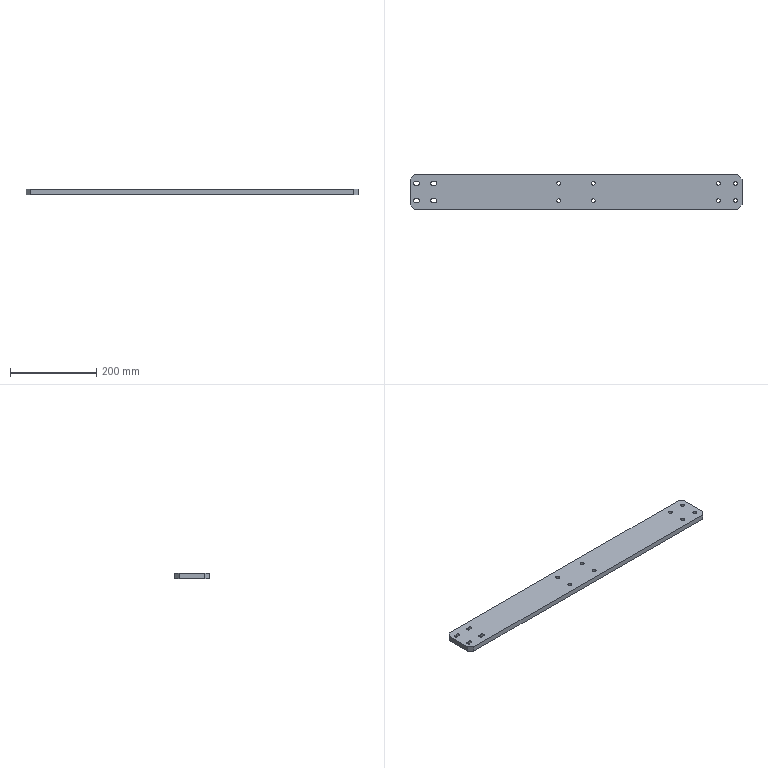Part | SolidWorks | features BaseBody 1 | 1 solid | 46 faces | box 770 x 80 x 12 mm | volume 725479 mm3 | cylinder 28 | plane 18 | commonest cylinder face diameters 9 x28
STEP:
#1=CARTESIAN_POINT('',(-363.,-20.,0.));
#2=VERTEX_POINT('',#1);
#3=CARTESIAN_POINT('',(-367.5,-15.5,0.));
#4=VERTEX_POINT('',#3);
#5=CARTESIAN_POINT('',(-367.5,-20.,0.));
#6=DIRECTION('',(0.,0.,1.));
#7=DIRECTION('',(1.,0.,0.));
#8=AXIS2_PLACEMENT_3D('',#5,#6,#7);
#9=CIRCLE('',#8,4.5);
#10=EDGE_CURVE('',#2,#4,#9,.T.);
#11=ORIENTED_EDGE('',*,*,#10,.F.);
#12=CARTESIAN_POINT('',(-363.,-20.,12.));
#13=VERTEX_POINT('',#12);
#14=CARTESIAN_POINT('',(-363.,-20.,0.));
#15=DIRECTION('',(0.,0.,1.));
#16=VECTOR('',#15,1000.);
#17=LINE('',#14,#16);
#18=EDGE_CURVE('',#2,#13,#17,.T.);
#19=ORIENTED_EDGE('',*,*,#18,.T.);
#20=CARTESIAN_POINT('',(-367.5,-15.5,12.));
#21=VERTEX_POINT('',#20);
#22=CARTESIAN_POINT('',(-367.5,-20.,12.));
#23=DIRECTION('',(0.,0.,1.));
#24=DIRECTION('',(1.,0.,0.));
#25=AXIS2_PLACEMENT_3D('',#22,#23,#24);
#26=CIRCLE('',#25,4.5);
#27=EDGE_CURVE('',#13,#21,#26,.T.);
#28=ORIENTED_EDGE('',*,*,#27,.T.);
#29=CARTESIAN_POINT('',(-367.5,-15.5,0.));
#30=DIRECTION('',(0.,0.,1.));
#31=VECTOR('',#30,1000.);
#32=LINE('',#29,#31);
#33=EDGE_CURVE('',#4,#21,#32,.T.);
#34=ORIENTED_EDGE('',*,*,#33,.F.);
#35=EDGE_LOOP('',(#11,#19,#28,#34));
#36=FACE_OUTER_BOUND('',#35,.T.);
#37=CARTESIAN_POINT('',(-367.5,-20.,0.));
#38=DIRECTION('',(0.,0.,1.));
#39=DIRECTION('',(1.,0.,0.));
#40=AXIS2_PLACEMENT_3D('',#37,#38,#39);
#41=CYLINDRICAL_SURFACE('',#40,4.5);
#42=ADVANCED_FACE('',(#36),#41,.F.);
#43=CARTESIAN_POINT('',(-323.,-20.,0.));
#44=VERTEX_POINT('',#43);
#45=CARTESIAN_POINT('',(-327.5,-15.5,0.));
#46=VERTEX_POINT('',#45);
#47=CARTESIAN_POINT('',(-327.5,-20.,0.));
#48=DIRECTION('',(0.,0.,1.));
#49=DIRECTION('',(1.,0.,0.));
#50=AXIS2_PLACEMENT_3D('',#47,#48,#49);
#51=CIRCLE('',#50,4.5);
#52=EDGE_CURVE('',#44,#46,#51,.T.);
#53=ORIENTED_EDGE('',*,*,#52,.F.);
#54=CARTESIAN_POINT('',(-323.,-20.,12.));
#55=VERTEX_POINT('',#54);
#56=CARTESIAN_POINT('',(-323.,-20.,0.));
#57=DIRECTION('',(0.,0.,1.));
#58=VECTOR('',#57,1000.);
#59=LINE('',#56,#58);
#60=EDGE_CURVE('',#44,#55,#59,.T.);
#61=ORIENTED_EDGE('',*,*,#60,.T.);
#62=CARTESIAN_POINT('',(-327.5,-15.5,12.));
#63=VERTEX_POINT('',#62);
#64=CARTESIAN_POINT('',(-327.5,-20.,12.));
#65=DIRECTION('',(0.,0.,1.));
#66=DIRECTION('',(1.,0.,0.));
#67=AXIS2_PLACEMENT_3D('',#64,#65,#66);
#68=CIRCLE('',#67,4.5);
#69=EDGE_CURVE('',#55,#63,#68,.T.);
#70=ORIENTED_EDGE('',*,*,#69,.T.);
#71=CARTESIAN_POINT('',(-327.5,-15.5,0.));
#72=DIRECTION('',(0.,0.,1.));
#73=VECTOR('',#72,1000.);
#74=LINE('',#71,#73);
#75=EDGE_CURVE('',#46,#63,#74,.T.);
#76=ORIENTED_EDGE('',*,*,#75,.F.);
#77=EDGE_LOOP('',(#53,#61,#70,#76));
#78=FACE_OUTER_BOUND('',#77,.T.);
#79=CARTESIAN_POINT('',(-327.5,-20.,0.));
#80=DIRECTION('',(0.,0.,1.));
#81=DIRECTION('',(1.,0.,0.));
#82=AXIS2_PLACEMENT_3D('',#79,#80,#81);
#83=CYLINDRICAL_SURFACE('',#82,4.5);
#84=ADVANCED_FACE('',(#78),#83,.F.);
#85=CARTESIAN_POINT('',(-323.,20.,0.));
#86=VERTEX_POINT('',#85);
#87=CARTESIAN_POINT('',(-327.5,24.5,0.));
#88=VERTEX_POINT('',#87);
#89=CARTESIAN_POINT('',(-327.5,20.,0.));
#90=DIRECTION('',(0.,0.,1.));
#91=DIRECTION('',(1.,0.,0.));
#92=AXIS2_PLACEMENT_3D('',#89,#90,#91);
#93=CIRCLE('',#92,4.5);
#94=EDGE_CURVE('',#86,#88,#93,.T.);
#95=ORIENTED_EDGE('',*,*,#94,.F.);
#96=CARTESIAN_POINT('',(-323.,20.,12.));
#97=VERTEX_POINT('',#96);
#98=CARTESIAN_POINT('',(-323.,20.,0.));
#99=DIRECTION('',(0.,0.,1.));
#100=VECTOR('',#99,1000.);
#101=LINE('',#98,#100);
#102=EDGE_CURVE('',#86,#97,#101,.T.);
#103=ORIENTED_EDGE('',*,*,#102,.T.);
#104=CARTESIAN_POINT('',(-327.5,24.5,12.));
#105=VERTEX_POINT('',#104);
#106=CARTESIAN_POINT('',(-327.5,20.,12.));
#107=DIRECTION('',(0.,0.,1.));
#108=DIRECTION('',(1.,0.,0.));
#109=AXIS2_PLACEMENT_3D('',#106,#107,#108);
#110=CIRCLE('',#109,4.5);
#111=EDGE_CURVE('',#97,#105,#110,.T.);
#112=ORIENTED_EDGE('',*,*,#111,.T.);
#113=CARTESIAN_POINT('',(-327.5,24.5,0.));
#114=DIRECTION('',(0.,0.,1.));
#115=VECTOR('',#114,1000.);
#116=LINE('',#113,#115);
#117=EDGE_CURVE('',#88,#105,#116,.T.);
#118=ORIENTED_EDGE('',*,*,#117,.F.);
#119=EDGE_LOOP('',(#95,#103,#112,#118));
#120=FACE_OUTER_BOUND('',#119,.T.);
#121=CARTESIAN_POINT('',(-327.5,20.,0.));
#122=DIRECTION('',(0.,0.,1.));
#123=DIRECTION('',(1.,0.,0.));
#124=AXIS2_PLACEMENT_3D('',#121,#122,#123);
#125=CYLINDRICAL_SURFACE('',#124,4.5);
#126=ADVANCED_FACE('',(#120),#125,.F.);
#127=CARTESIAN_POINT('',(-363.,20.,0.));
#128=VERTEX_POINT('',#127);
#129=CARTESIAN_POINT('',(-367.5,24.5,0.));
#130=VERTEX_POINT('',#129);
#131=CARTESIAN_POINT('',(-367.5,20.,0.));
#132=DIRECTION('',(0.,0.,1.));
#133=DIRECTION('',(1.,0.,0.));
#134=AXIS2_PLACEMENT_3D('',#131,#132,#133);
#135=CIRCLE('',#134,4.5);
#136=EDGE_CURVE('',#128,#130,#135,.T.);
#137=ORIENTED_EDGE('',*,*,#136,.F.);
#138=CARTESIAN_POINT('',(-363.,20.,12.));
#139=VERTEX_POINT('',#138);
#140=CARTESIAN_POINT('',(-363.,20.,0.));
#141=DIRECTION('',(0.,0.,1.));
#142=VECTOR('',#141,1000.);
#143=LINE('',#140,#142);
#144=EDGE_CURVE('',#128,#139,#143,.T.);
#145=ORIENTED_EDGE('',*,*,#144,.T.);
#146=CARTESIAN_POINT('',(-367.5,24.5,12.));
#147=VERTEX_POINT('',#146);
#148=CARTESIAN_POINT('',(-367.5,20.,12.));
#149=DIRECTION('',(0.,0.,1.));
#150=DIRECTION('',(1.,0.,0.));
#151=AXIS2_PLACEMENT_3D('',#148,#149,#150);
#152=CIRCLE('',#151,4.5);
#153=EDGE_CURVE('',#139,#147,#152,.T.);
#154=ORIENTED_EDGE('',*,*,#153,.T.);
#155=CARTESIAN_POINT('',(-367.5,24.5,0.));
#156=DIRECTION('',(0.,0.,1.));
#157=VECTOR('',#156,1000.);
#158=LINE('',#155,#157);
#159=EDGE_CURVE('',#130,#147,#158,.T.);
#160=ORIENTED_EDGE('',*,*,#159,.F.);
#161=EDGE_LOOP('',(#137,#145,#154,#160));
#162=FACE_OUTER_BOUND('',#161,.T.);
#163=CARTESIAN_POINT('',(-367.5,20.,0.));
#164=DIRECTION('',(0.,0.,1.));
#165=DIRECTION('',(1.,0.,0.));
#166=AXIS2_PLACEMENT_3D('',#163,#164,#165);
#167=CYLINDRICAL_SURFACE('',#166,4.5);
#168=ADVANCED_FACE('',(#162),#167,.F.);
#169=CARTESIAN_POINT('',(334.5,20.,0.));
#170=VERTEX_POINT('',#169);
#171=CARTESIAN_POINT('',(325.5,20.,0.));
#172=VERTEX_POINT('',#171);
#173=CARTESIAN_POINT('',(330.,20.,0.));
#174=DIRECTION('',(0.,0.,-1.));
#175=DIRECTION('',(-1.,0.,0.));
#176=AXIS2_PLACEMENT_3D('',#173,#174,#175);
#177=CIRCLE('',#176,4.5);
#178=EDGE_CURVE('',#170,#172,#177,.T.);
#179=ORIENTED_EDGE('',*,*,#178,.T.);
#180=CARTESIAN_POINT('',(325.5,20.,12.));
#181=VERTEX_POINT('',#180);
#182=CARTESIAN_POINT('',(325.5,20.,12.));
#183=DIRECTION('',(0.,0.,1.));
#184=VECTOR('',#183,1000.);
#185=LINE('',#182,#184);
#186=EDGE_CURVE('',#172,#181,#185,.T.);
#187=ORIENTED_EDGE('',*,*,#186,.T.);
#188=CARTESIAN_POINT('',(334.5,20.,12.));
#189=VERTEX_POINT('',#188);
#190=CARTESIAN_POINT('',(330.,20.,12.));
#191=DIRECTION('',(0.,0.,1.));
#192=DIRECTION('',(1.,0.,0.));
#193=AXIS2_PLACEMENT_3D('',#190,#191,#192);
#194=CIRCLE('',#193,4.5);
#195=EDGE_CURVE('',#181,#189,#194,.T.);
#196=ORIENTED_EDGE('',*,*,#195,.T.);
#197=CARTESIAN_POINT('',(334.5,20.,12.));
#198=DIRECTION('',(0.,0.,1.));
#199=VECTOR('',#198,1000.);
#200=LINE('',#197,#199);
#201=EDGE_CURVE('',#170,#189,#200,.T.);
#202=ORIENTED_EDGE('',*,*,#201,.F.);
#203=EDGE_LOOP('',(#179,#187,#196,#202));
#204=FACE_OUTER_BOUND('',#203,.T.);
#205=CARTESIAN_POINT('',(330.,20.,12.));
#206=DIRECTION('',(0.,0.,1.));
#207=DIRECTION('',(1.,0.,0.));
#208=AXIS2_PLACEMENT_3D('',#205,#206,#207);
#209=CYLINDRICAL_SURFACE('',#208,4.5);
#210=ADVANCED_FACE('',(#204),#209,.F.);
#211=CARTESIAN_POINT('',(374.5,20.,0.));
#212=VERTEX_POINT('',#211);
#213=CARTESIAN_POINT('',(365.5,20.,0.));
#214=VERTEX_POINT('',#213);
#215=CARTESIAN_POINT('',(370.,20.,0.));
#216=DIRECTION('',(0.,0.,-1.));
#217=DIRECTION('',(-1.,0.,0.));
#218=AXIS2_PLACEMENT_3D('',#215,#216,#217);
#219=CIRCLE('',#218,4.5);
#220=EDGE_CURVE('',#212,#214,#219,.T.);
#221=ORIENTED_EDGE('',*,*,#220,.T.);
#222=CARTESIAN_POINT('',(365.5,20.,12.));
#223=VERTEX_POINT('',#222);
#224=CARTESIAN_POINT('',(365.5,20.,12.));
#225=DIRECTION('',(0.,0.,1.));
#226=VECTOR('',#225,1000.);
#227=LINE('',#224,#226);
#228=EDGE_CURVE('',#214,#223,#227,.T.);
#229=ORIENTED_EDGE('',*,*,#228,.T.);
#230=CARTESIAN_POINT('',(374.5,20.,12.));
#231=VERTEX_POINT('',#230);
#232=CARTESIAN_POINT('',(370.,20.,12.));
#233=DIRECTION('',(0.,0.,1.));
#234=DIRECTION('',(1.,0.,0.));
#235=AXIS2_PLACEMENT_3D('',#232,#233,#234);
#236=CIRCLE('',#235,4.5);
#237=EDGE_CURVE('',#223,#231,#236,.T.);
#238=ORIENTED_EDGE('',*,*,#237,.T.);
#239=CARTESIAN_POINT('',(374.5,20.,12.));
#240=DIRECTION('',(0.,0.,1.));
#241=VECTOR('',#240,1000.);
#242=LINE('',#239,#241);
#243=EDGE_CURVE('',#212,#231,#242,.T.);
#244=ORIENTED_EDGE('',*,*,#243,.F.);
#245=EDGE_LOOP('',(#221,#229,#238,#244));
#246=FACE_OUTER_BOUND('',#245,.T.);
#247=CARTESIAN_POINT('',(370.,20.,12.));
#248=DIRECTION('',(0.,0.,1.));
#249=DIRECTION('',(1.,0.,0.));
#250=AXIS2_PLACEMENT_3D('',#247,#248,#249);
#251=CYLINDRICAL_SURFACE('',#250,4.5);
#252=ADVANCED_FACE('',(#246),#251,.F.);
#253=CARTESIAN_POINT('',(374.5,-20.,0.));
#254=VERTEX_POINT('',#253);
#255=CARTESIAN_POINT('',(365.5,-20.,0.));
#256=VERTEX_POINT('',#255);
#257=CARTESIAN_POINT('',(370.,-20.,0.));
#258=DIRECTION('',(0.,0.,-1.));
#259=DIRECTION('',(-1.,0.,0.));
#260=AXIS2_PLACEMENT_3D('',#257,#258,#259);
#261=CIRCLE('',#260,4.5);
#262=EDGE_CURVE('',#254,#256,#261,.T.);
#263=ORIENTED_EDGE('',*,*,#262,.T.);
#264=CARTESIAN_POINT('',(365.5,-20.,12.));
#265=VERTEX_POINT('',#264);
#266=CARTESIAN_POINT('',(365.5,-20.,12.));
#267=DIRECTION('',(0.,0.,1.));
#268=VECTOR('',#267,1000.);
#269=LINE('',#266,#268);
#270=EDGE_CURVE('',#256,#265,#269,.T.);
#271=ORIENTED_EDGE('',*,*,#270,.T.);
#272=CARTESIAN_POINT('',(374.5,-20.,12.));
#273=VERTEX_POINT('',#272);
#274=CARTESIAN_POINT('',(370.,-20.,12.));
#275=DIRECTION('',(0.,0.,1.));
#276=DIRECTION('',(1.,0.,0.));
#277=AXIS2_PLACEMENT_3D('',#274,#275,#276);
#278=CIRCLE('',#277,4.5);
#279=EDGE_CURVE('',#265,#273,#278,.T.);
#280=ORIENTED_EDGE('',*,*,#279,.T.);
#281=CARTESIAN_POINT('',(374.5,-20.,12.));
#282=DIRECTION('',(0.,0.,1.));
#283=VECTOR('',#282,1000.);
#284=LINE('',#281,#283);
#285=EDGE_CURVE('',#254,#273,#284,.T.);
#286=ORIENTED_EDGE('',*,*,#285,.F.);
#287=EDGE_LOOP('',(#263,#271,#280,#286));
#288=FACE_OUTER_BOUND('',#287,.T.);
#289=CARTESIAN_POINT('',(370.,-20.,12.));
#290=DIRECTION('',(0.,0.,1.));
#291=DIRECTION('',(1.,0.,0.));
#292=AXIS2_PLACEMENT_3D('',#289,#290,#291);
#293=CYLINDRICAL_SURFACE('',#292,4.5);
#294=ADVANCED_FACE('',(#288),#293,.F.);
#295=CARTESIAN_POINT('',(334.5,-20.,0.));
#296=VERTEX_POINT('',#295);
#297=CARTESIAN_POINT('',(325.5,-20.,0.));
#298=VERTEX_POINT('',#297);
#299=CARTESIAN_POINT('',(330.,-20.,0.));
#300=DIRECTION('',(0.,0.,-1.));
#301=DIRECTION('',(-1.,0.,0.));
#302=AXIS2_PLACEMENT_3D('',#299,#300,#301);
#303=CIRCLE('',#302,4.5);
#304=EDGE_CURVE('',#296,#298,#303,.T.);
#305=ORIENTED_EDGE('',*,*,#304,.T.);
#306=CARTESIAN_POINT('',(325.5,-20.,12.));
#307=VERTEX_POINT('',#306);
#308=CARTESIAN_POINT('',(325.5,-20.,12.));
#309=DIRECTION('',(0.,0.,1.));
#310=VECTOR('',#309,1000.);
#311=LINE('',#308,#310);
#312=EDGE_CURVE('',#298,#307,#311,.T.);
#313=ORIENTED_EDGE('',*,*,#312,.T.);
#314=CARTESIAN_POINT('',(334.5,-20.,12.));
#315=VERTEX_POINT('',#314);
#316=CARTESIAN_POINT('',(330.,-20.,12.));
#317=DIRECTION('',(0.,0.,1.));
#318=DIRECTION('',(1.,0.,0.));
#319=AXIS2_PLACEMENT_3D('',#316,#317,#318);
#320=CIRCLE('',#319,4.5);
#321=EDGE_CURVE('',#307,#315,#320,.T.);
#322=ORIENTED_EDGE('',*,*,#321,.T.);
#323=CARTESIAN_POINT('',(334.5,-20.,12.));
#324=DIRECTION('',(0.,0.,1.));
#325=VECTOR('',#324,1000.);
#326=LINE('',#323,#325);
#327=EDGE_CURVE('',#296,#315,#326,.T.);
#328=ORIENTED_EDGE('',*,*,#327,.F.);
#329=EDGE_LOOP('',(#305,#313,#322,#328));
#330=FACE_OUTER_BOUND('',#329,.T.);
#331=CARTESIAN_POINT('',(330.,-20.,12.));
#332=DIRECTION('',(0.,0.,1.));
#333=DIRECTION('',(1.,0.,0.));
#334=AXIS2_PLACEMENT_3D('',#331,#332,#333);
#335=CYLINDRICAL_SURFACE('',#334,4.5);
#336=ADVANCED_FACE('',(#330),#335,.F.);
#337=CARTESIAN_POINT('',(44.5,-20.,0.));
#338=VERTEX_POINT('',#337);
#339=CARTESIAN_POINT('',(35.5,-20.,0.));
#340=VERTEX_POINT('',#339);
#341=CARTESIAN_POINT('',(40.,-20.,0.));
#342=DIRECTION('',(0.,0.,-1.));
#343=DIRECTION('',(-1.,0.,0.));
#344=AXIS2_PLACEMENT_3D('',#341,#342,#343);
#345=CIRCLE('',#344,4.5);
#346=EDGE_CURVE('',#338,#340,#345,.T.);
#347=ORIENTED_EDGE('',*,*,#346,.T.);
#348=CARTESIAN_POINT('',(35.5,-20.,12.));
#349=VERTEX_POINT('',#348);
#350=CARTESIAN_POINT('',(35.5,-20.,12.));
#351=DIRECTION('',(0.,0.,1.));
#352=VECTOR('',#351,1000.);
#353=LINE('',#350,#352);
#354=EDGE_CURVE('',#340,#349,#353,.T.);
#355=ORIENTED_EDGE('',*,*,#354,.T.);
#356=CARTESIAN_POINT('',(44.5,-20.,12.));
#357=VERTEX_POINT('',#356);
#358=CARTESIAN_POINT('',(40.,-20.,12.));
#359=DIRECTION('',(0.,0.,1.));
#360=DIRECTION('',(1.,0.,0.));
#361=AXIS2_PLACEMENT_3D('',#358,#359,#360);
#362=CIRCLE('',#361,4.5);
#363=EDGE_CURVE('',#349,#357,#362,.T.);
#364=ORIENTED_EDGE('',*,*,#363,.T.);
#365=CARTESIAN_POINT('',(44.5,-20.,12.));
#366=DIRECTION('',(0.,0.,1.));
#367=VECTOR('',#366,1000.);
#368=LINE('',#365,#367);
#369=EDGE_CURVE('',#338,#357,#368,.T.);
#370=ORIENTED_EDGE('',*,*,#369,.F.);
#371=EDGE_LOOP('',(#347,#355,#364,#370));
#372=FACE_OUTER_BOUND('',#371,.T.);
#373=CARTESIAN_POINT('',(40.,-20.,12.));
#374=DIRECTION('',(0.,0.,1.));
#375=DIRECTION('',(1.,0.,0.));
#376=AXIS2_PLACEMENT_3D('',#373,#374,#375);
#377=CYLINDRICAL_SURFACE('',#376,4.5);
#378=ADVANCED_FACE('',(#372),#377,.F.);
#379=CARTESIAN_POINT('',(-35.5,20.,0.));
#380=VERTEX_POINT('',#379);
#381=CARTESIAN_POINT('',(-44.5,20.,0.));
#382=VERTEX_POINT('',#381);
#383=CARTESIAN_POINT('',(-40.,20.,0.));
#384=DIRECTION('',(0.,0.,-1.));
#385=DIRECTION('',(-1.,0.,0.));
#386=AXIS2_PLACEMENT_3D('',#383,#384,#385);
#387=CIRCLE('',#386,4.5);
#388=EDGE_CURVE('',#380,#382,#387,.T.);
#389=ORIENTED_EDGE('',*,*,#388,.T.);
#390=CARTESIAN_POINT('',(-44.5,20.,12.));
#391=VERTEX_POINT('',#390);
#392=CARTESIAN_POINT('',(-44.5,20.,12.));
#393=DIRECTION('',(0.,0.,1.));
#394=VECTOR('',#393,1000.);
#395=LINE('',#392,#394);
#396=EDGE_CURVE('',#382,#391,#395,.T.);
#397=ORIENTED_EDGE('',*,*,#396,.T.);
#398=CARTESIAN_POINT('',(-35.5,20.,12.));
#399=VERTEX_POINT('',#398);
#400=CARTESIAN_POINT('',(-40.,20.,12.));
#401=DIRECTION('',(0.,0.,1.));
#402=DIRECTION('',(1.,0.,0.));
#403=AXIS2_PLACEMENT_3D('',#400,#401,#402);
#404=CIRCLE('',#403,4.5);
#405=EDGE_CURVE('',#391,#399,#404,.T.);
#406=ORIENTED_EDGE('',*,*,#405,.T.);
#407=CARTESIAN_POINT('',(-35.5,20.,12.));
#408=DIRECTION('',(0.,0.,1.));
#409=VECTOR('',#408,1000.);
#410=LINE('',#407,#409);
#411=EDGE_CURVE('',#380,#399,#410,.T.);
#412=ORIENTED_EDGE('',*,*,#411,.F.);
#413=EDGE_LOOP('',(#389,#397,#406,#412));
#414=FACE_OUTER_BOUND('',#413,.T.);
#415=CARTESIAN_POINT('',(-40.,20.,12.));
#416=DIRECTION('',(0.,0.,1.));
#417=DIRECTION('',(1.,0.,0.));
#418=AXIS2_PLACEMENT_3D('',#415,#416,#417);
#419=CYLINDRICAL_SURFACE('',#418,4.5);
#420=ADVANCED_FACE('',(#414),#419,.F.);
#421=CARTESIAN_POINT('',(-35.5,-20.,0.));
#422=VERTEX_POINT('',#421);
#423=CARTESIAN_POINT('',(-44.5,-20.,0.));
#424=VERTEX_POINT('',#423);
#425=CARTESIAN_POINT('',(-40.,-20.,0.));
#426=DIRECTION('',(0.,0.,-1.));
#427=DIRECTION('',(-1.,0.,0.));
#428=AXIS2_PLACEMENT_3D('',#425,#426,#427);
#429=CIRCLE('',#428,4.5);
#430=EDGE_CURVE('',#422,#424,#429,.T.);
#431=ORIENTED_EDGE('',*,*,#430,.T.);
#432=CARTESIAN_POINT('',(-44.5,-20.,12.));
#433=VERTEX_POINT('',#432);
#434=CARTESIAN_POINT('',(-44.5,-20.,12.));
#435=DIRECTION('',(0.,0.,1.));
#436=VECTOR('',#435,1000.);
#437=LINE('',#434,#436);
#438=EDGE_CURVE('',#424,#433,#437,.T.);
#439=ORIENTED_EDGE('',*,*,#438,.T.);
#440=CARTESIAN_POINT('',(-35.5,-20.,12.));
#441=VERTEX_POINT('',#440);
#442=CARTESIAN_POINT('',(-40.,-20.,12.));
#443=DIRECTION('',(0.,0.,1.));
#444=DIRECTION('',(1.,0.,0.));
#445=AXIS2_PLACEMENT_3D('',#442,#443,#444);
#446=CIRCLE('',#445,4.5);
#447=EDGE_CURVE('',#433,#441,#446,.T.);
#448=ORIENTED_EDGE('',*,*,#447,.T.);
#449=CARTESIAN_POINT('',(-35.5,-20.,12.));
#450=DIRECTION('',(0.,0.,1.));
#451=VECTOR('',#450,1000.);
#452=LINE('',#449,#451);
#453=EDGE_CURVE('',#422,#441,#452,.T.);
#454=ORIENTED_EDGE('',*,*,#453,.F.);
#455=EDGE_LOOP('',(#431,#439,#448,#454));
#456=FACE_OUTER_BOUND('',#455,.T.);
#457=CARTESIAN_POINT('',(-40.,-20.,12.));
#458=DIRECTION('',(0.,0.,1.));
#459=DIRECTION('',(1.,0.,0.));
#460=AXIS2_PLACEMENT_3D('',#457,#458,#459);
#461=CYLINDRICAL_SURFACE('',#460,4.5);
#462=ADVANCED_FACE('',(#456),#461,.F.);
#463=CARTESIAN_POINT('',(44.5,20.,0.));
#464=VERTEX_POINT('',#463);
#465=CARTESIAN_POINT('',(35.5,20.,0.));
#466=VERTEX_POINT('',#465);
#467=CARTESIAN_POINT('',(40.,20.,0.));
#468=DIRECTION('',(0.,0.,-1.));
#469=DIRECTION('',(-1.,0.,0.));
#470=AXIS2_PLACEMENT_3D('',#467,#468,#469);
#471=CIRCLE('',#470,4.5);
#472=EDGE_CURVE('',#464,#466,#471,.T.);
#473=ORIENTED_EDGE('',*,*,#472,.T.);
#474=CARTESIAN_POINT('',(35.5,20.,12.));
#475=VERTEX_POINT('',#474);
#476=CARTESIAN_POINT('',(35.5,20.,12.));
#477=DIRECTION('',(0.,0.,1.));
#478=VECTOR('',#477,1000.);
#479=LINE('',#476,#478);
#480=EDGE_CURVE('',#466,#475,#479,.T.);
#481=ORIENTED_EDGE('',*,*,#480,.T.);
#482=CARTESIAN_POINT('',(44.5,20.,12.));
#483=VERTEX_POINT('',#482);
#484=CARTESIAN_POINT('',(40.,20.,12.));
#485=DIRECTION('',(0.,0.,1.));
#486=DIRECTION('',(1.,0.,0.));
#487=AXIS2_PLACEMENT_3D('',#484,#485,#486);
#488=CIRCLE('',#487,4.5);
#489=EDGE_CURVE('',#475,#483,#488,.T.);
#490=ORIENTED_EDGE('',*,*,#489,.T.);
#491=CARTESIAN_POINT('',(44.5,20.,12.));
#492=DIRECTION('',(0.,0.,1.));
#493=VECTOR('',#492,1000.);
#494=LINE('',#491,#493);
#495=EDGE_CURVE('',#464,#483,#494,.T.);
#496=ORIENTED_EDGE('',*,*,#495,.F.);
#497=EDGE_LOOP('',(#473,#481,#490,#496));
#498=FACE_OUTER_BOUND('',#497,.T.);
#499=CARTESIAN_POINT('',(40.,20.,12.));
#500=DIRECTION('',(0.,0.,1.));
#501=DIRECTION('',(1.,0.,0.));
#502=AXIS2_PLACEMENT_3D('',#499,#500,#501);
#503=CYLINDRICAL_SURFACE('',#502,4.5);
#504=ADVANCED_FACE('',(#498),#503,.F.);
#505=CARTESIAN_POINT('',(375.,40.,0.));
#506=VERTEX_POINT('',#505);
#507=CARTESIAN_POINT('',(-375.,40.,0.));
#508=VERTEX_POINT('',#507);
#509=CARTESIAN_POINT('',(-375.,40.,0.));
#510=DIRECTION('',(-1.,0.,0.));
#511=VECTOR('',#510,1000.);
#512=LINE('',#509,#511);
#513=EDGE_CURVE('',#506,#508,#512,.T.);
#514=ORIENTED_EDGE('',*,*,#513,.T.);
#515=CARTESIAN_POINT('',(-375.,40.,12.));
#516=VERTEX_POINT('',#515);
#517=CARTESIAN_POINT('',(-375.,40.,12.));
#518=DIRECTION('',(0.,0.,-1.));
#519=VECTOR('',#518,1000.);
#520=LINE('',#517,#519);
#521=EDGE_CURVE('',#516,#508,#520,.T.);
#522=ORIENTED_EDGE('',*,*,#521,.F.);
#523=CARTESIAN_POINT('',(375.,40.,12.));
#524=VERTEX_POINT('',#523);
#525=CARTESIAN_POINT('',(-375.,40.,12.));
#526=DIRECTION('',(-1.,0.,0.));
#527=VECTOR('',#526,1000.);
#528=LINE('',#525,#527);
#529=EDGE_CURVE('',#524,#516,#528,.T.);
#530=ORIENTED_EDGE('',*,*,#529,.F.);
#531=CARTESIAN_POINT('',(375.,40.,12.));
#532=DIRECTION('',(0.,0.,-1.));
#533=VECTOR('',#532,1000.);
#534=LINE('',#531,#533);
#535=EDGE_CURVE('',#524,#506,#534,.T.);
#536=ORIENTED_EDGE('',*,*,#535,.T.);
#537=EDGE_LOOP('',(#514,#522,#530,#536));
#538=FACE_OUTER_BOUND('',#537,.T.);
#539=CARTESIAN_POINT('',(-375.,40.,12.));
#540=DIRECTION('',(0.,-1.,0.));
#541=DIRECTION('',(0.,0.,-1.));
#542=AXIS2_PLACEMENT_3D('',#539,#540,#541);
#543=PLANE('',#542);
#544=ADVANCED_FACE('',(#538),#543,.F.);
#545=CARTESIAN_POINT('',(-385.,30.,0.));
#546=VERTEX_POINT('',#545);
#547=CARTESIAN_POINT('',(-385.,30.,0.));
#548=DIRECTION('',(-0.7071,-0.7071,0.));
#549=VECTOR('',#548,1000.);
#550=LINE('',#547,#549);
#551=EDGE_CURVE('',#508,#546,#550,.T.);
#552=ORIENTED_EDGE('',*,*,#551,.T.);
#553=CARTESIAN_POINT('',(-385.,30.,12.));
#554=VERTEX_POINT('',#553);
#555=CARTESIAN_POINT('',(-385.,30.,12.));
#556=DIRECTION('',(0.,0.,-1.));
#557=VECTOR('',#556,1000.);
#558=LINE('',#555,#557);
#559=EDGE_CURVE('',#554,#546,#558,.T.);
#560=ORIENTED_EDGE('',*,*,#559,.F.);
#561=CARTESIAN_POINT('',(-385.,30.,12.));
#562=DIRECTION('',(-0.7071,-0.7071,0.));
#563=VECTOR('',#562,1000.);
#564=LINE('',#561,#563);
#565=EDGE_CURVE('',#516,#554,#564,.T.);
#566=ORIENTED_EDGE('',*,*,#565,.F.);
#567=ORIENTED_EDGE('',*,*,#521,.T.);
#568=EDGE_LOOP('',(#552,#560,#566,#567));
#569=FACE_OUTER_BOUND('',#568,.T.);
#570=CARTESIAN_POINT('',(-385.,30.,12.));
#571=DIRECTION('',(0.7071,-0.7071,0.));
#572=DIRECTION('',(0.7071,0.7071,0.));
#573=AXIS2_PLACEMENT_3D('',#570,#571,#572);
#574=PLANE('',#573);
#575=ADVANCED_FACE('',(#569),#574,.F.);
#576=CARTESIAN_POINT('',(-385.,-30.,0.));
#577=VERTEX_POINT('',#576);
#578=CARTESIAN_POINT('',(-385.,30.,0.));
#579=DIRECTION('',(0.,-1.,0.));
#580=VECTOR('',#579,1000.);
#581=LINE('',#578,#580);
#582=EDGE_CURVE('',#546,#577,#581,.T.);
#583=ORIENTED_EDGE('',*,*,#582,.T.);
#584=CARTESIAN_POINT('',(-385.,-30.,12.));
#585=VERTEX_POINT('',#584);
#586=CARTESIAN_POINT('',(-385.,-30.,12.));
#587=DIRECTION('',(0.,0.,-1.));
#588=VECTOR('',#587,1000.);
#589=LINE('',#586,#588);
#590=EDGE_CURVE('',#585,#577,#589,.T.);
#591=ORIENTED_EDGE('',*,*,#590,.F.);
#592=CARTESIAN_POINT('',(-385.,30.,12.));
#593=DIRECTION('',(0.,-1.,0.));
#594=VECTOR('',#593,1000.);
#595=LINE('',#592,#594);
#596=EDGE_CURVE('',#554,#585,#595,.T.);
#597=ORIENTED_EDGE('',*,*,#596,.F.);
#598=ORIENTED_EDGE('',*,*,#559,.T.);
#599=EDGE_LOOP('',(#583,#591,#597,#598));
#600=FACE_OUTER_BOUND('',#599,.T.);
#601=CARTESIAN_POINT('',(-385.,30.,12.));
#602=DIRECTION('',(1.,0.,0.));
#603=DIRECTION('',(0.,0.,-1.));
#604=AXIS2_PLACEMENT_3D('',#601,#602,#603);
#605=PLANE('',#604);
#606=ADVANCED_FACE('',(#600),#605,.F.);
#607=CARTESIAN_POINT('',(-375.,-40.,0.));
#608=VERTEX_POINT('',#607);
#609=CARTESIAN_POINT('',(-385.,-30.,0.));
#610=DIRECTION('',(0.7071,-0.7071,0.));
#611=VECTOR('',#610,1000.);
#612=LINE('',#609,#611);
#613=EDGE_CURVE('',#577,#608,#612,.T.);
#614=ORIENTED_EDGE('',*,*,#613,.T.);
#615=CARTESIAN_POINT('',(-375.,-40.,12.));
#616=VERTEX_POINT('',#615);
#617=CARTESIAN_POINT('',(-375.,-40.,12.));
#618=DIRECTION('',(0.,0.,-1.));
#619=VECTOR('',#618,1000.);
#620=LINE('',#617,#619);
#621=EDGE_CURVE('',#616,#608,#620,.T.);
#622=ORIENTED_EDGE('',*,*,#621,.F.);
#623=CARTESIAN_POINT('',(-385.,-30.,12.));
#624=DIRECTION('',(0.7071,-0.7071,0.));
#625=VECTOR('',#624,1000.);
#626=LINE('',#623,#625);
#627=EDGE_CURVE('',#585,#616,#626,.T.);
#628=ORIENTED_EDGE('',*,*,#627,.F.);
#629=ORIENTED_EDGE('',*,*,#590,.T.);
#630=EDGE_LOOP('',(#614,#622,#628,#629));
#631=FACE_OUTER_BOUND('',#630,.T.);
#632=CARTESIAN_POINT('',(-385.,-30.,12.));
#633=DIRECTION('',(0.7071,0.7071,0.));
#634=DIRECTION('',(-0.7071,0.7071,0.));
#635=AXIS2_PLACEMENT_3D('',#632,#633,#634);
#636=PLANE('',#635);
#637=ADVANCED_FACE('',(#631),#636,.F.);
#638=CARTESIAN_POINT('',(375.,-40.,0.));
#639=VERTEX_POINT('',#638);
#640=CARTESIAN_POINT('',(-375.,-40.,0.));
#641=DIRECTION('',(1.,0.,0.));
#642=VECTOR('',#641,1000.);
#643=LINE('',#640,#642);
#644=EDGE_CURVE('',#608,#639,#643,.T.);
#645=ORIENTED_EDGE('',*,*,#644,.T.);
#646=CARTESIAN_POINT('',(375.,-40.,12.));
#647=VERTEX_POINT('',#646);
#648=CARTESIAN_POINT('',(375.,-40.,12.));
#649=DIRECTION('',(0.,0.,-1.));
#650=VECTOR('',#649,1000.);
#651=LINE('',#648,#650);
#652=EDGE_CURVE('',#647,#639,#651,.T.);
#653=ORIENTED_EDGE('',*,*,#652,.F.);
#654=CARTESIAN_POINT('',(-375.,-40.,12.));
#655=DIRECTION('',(1.,0.,0.));
#656=VECTOR('',#655,1000.);
#657=LINE('',#654,#656);
#658=EDGE_CURVE('',#616,#647,#657,.T.);
#659=ORIENTED_EDGE('',*,*,#658,.F.);
#660=ORIENTED_EDGE('',*,*,#621,.T.);
#661=EDGE_LOOP('',(#645,#653,#659,#660));
#662=FACE_OUTER_BOUND('',#661,.T.);
#663=CARTESIAN_POINT('',(-375.,-40.,12.));
#664=DIRECTION('',(0.,1.,0.));
#665=DIRECTION('',(0.,0.,1.));
#666=AXIS2_PLACEMENT_3D('',#663,#664,#665);
#667=PLANE('',#666);
#668=ADVANCED_FACE('',(#662),#667,.F.);
#669=CARTESIAN_POINT('',(385.,-30.,0.));
#670=VERTEX_POINT('',#669);
#671=CARTESIAN_POINT('',(375.,-40.,0.));
#672=DIRECTION('',(0.7071,0.7071,0.));
#673=VECTOR('',#672,1000.);
#674=LINE('',#671,#673);
#675=EDGE_CURVE('',#639,#670,#674,.T.);
#676=ORIENTED_EDGE('',*,*,#675,.T.);
#677=CARTESIAN_POINT('',(385.,-30.,12.));
#678=VERTEX_POINT('',#677);
#679=CARTESIAN_POINT('',(385.,-30.,12.));
#680=DIRECTION('',(0.,0.,-1.));
#681=VECTOR('',#680,1000.);
#682=LINE('',#679,#681);
#683=EDGE_CURVE('',#678,#670,#682,.T.);
#684=ORIENTED_EDGE('',*,*,#683,.F.);
#685=CARTESIAN_POINT('',(375.,-40.,12.));
#686=DIRECTION('',(0.7071,0.7071,0.));
#687=VECTOR('',#686,1000.);
#688=LINE('',#685,#687);
#689=EDGE_CURVE('',#647,#678,#688,.T.);
#690=ORIENTED_EDGE('',*,*,#689,.F.);
#691=ORIENTED_EDGE('',*,*,#652,.T.);
#692=EDGE_LOOP('',(#676,#684,#690,#691));
#693=FACE_OUTER_BOUND('',#692,.T.);
#694=CARTESIAN_POINT('',(375.,-40.,12.));
#695=DIRECTION('',(-0.7071,0.7071,0.));
#696=DIRECTION('',(-0.7071,-0.7071,0.));
#697=AXIS2_PLACEMENT_3D('',#694,#695,#696);
#698=PLANE('',#697);
#699=ADVANCED_FACE('',(#693),#698,.F.);
#700=CARTESIAN_POINT('',(385.,30.,0.));
#701=VERTEX_POINT('',#700);
#702=CARTESIAN_POINT('',(385.,30.,0.));
#703=DIRECTION('',(0.,1.,0.));
#704=VECTOR('',#703,1000.);
#705=LINE('',#702,#704);
#706=EDGE_CURVE('',#670,#701,#705,.T.);
#707=ORIENTED_EDGE('',*,*,#706,.T.);
#708=CARTESIAN_POINT('',(385.,30.,12.));
#709=VERTEX_POINT('',#708);
#710=CARTESIAN_POINT('',(385.,30.,12.));
#711=DIRECTION('',(0.,0.,-1.));
#712=VECTOR('',#711,1000.);
#713=LINE('',#710,#712);
#714=EDGE_CURVE('',#709,#701,#713,.T.);
#715=ORIENTED_EDGE('',*,*,#714,.F.);
#716=CARTESIAN_POINT('',(385.,30.,12.));
#717=DIRECTION('',(0.,1.,0.));
#718=VECTOR('',#717,1000.);
#719=LINE('',#716,#718);
#720=EDGE_CURVE('',#678,#709,#719,.T.);
#721=ORIENTED_EDGE('',*,*,#720,.F.);
#722=ORIENTED_EDGE('',*,*,#683,.T.);
#723=EDGE_LOOP('',(#707,#715,#721,#722));
#724=FACE_OUTER_BOUND('',#723,.T.);
#725=CARTESIAN_POINT('',(385.,30.,12.));
#726=DIRECTION('',(-1.,0.,0.));
#727=DIRECTION('',(0.,0.,1.));
#728=AXIS2_PLACEMENT_3D('',#725,#726,#727);
#729=PLANE('',#728);
#730=ADVANCED_FACE('',(#724),#729,.F.);
#731=CARTESIAN_POINT('',(375.,40.,0.));
#732=DIRECTION('',(-0.7071,0.7071,0.));
#733=VECTOR('',#732,1000.);
#734=LINE('',#731,#733);
#735=EDGE_CURVE('',#701,#506,#734,.T.);
#736=ORIENTED_EDGE('',*,*,#735,.T.);
#737=ORIENTED_EDGE('',*,*,#535,.F.);
#738=CARTESIAN_POINT('',(375.,40.,12.));
#739=DIRECTION('',(-0.7071,0.7071,0.));
#740=VECTOR('',#739,1000.);
#741=LINE('',#738,#740);
#742=EDGE_CURVE('',#709,#524,#741,.T.);
#743=ORIENTED_EDGE('',*,*,#742,.F.);
#744=ORIENTED_EDGE('',*,*,#714,.T.);
#745=EDGE_LOOP('',(#736,#737,#743,#744));
#746=FACE_OUTER_BOUND('',#745,.T.);
#747=CARTESIAN_POINT('',(375.,40.,12.));
#748=DIRECTION('',(-0.7071,-0.7071,0.));
#749=DIRECTION('',(0.7071,-0.7071,0.));
#750=AXIS2_PLACEMENT_3D('',#747,#748,#749);
#751=PLANE('',#750);
#752=ADVANCED_FACE('',(#746),#751,.F.);
#753=CARTESIAN_POINT('',(330.,20.,12.));
#754=DIRECTION('',(0.,0.,1.));
#755=DIRECTION('',(1.,0.,0.));
#756=AXIS2_PLACEMENT_3D('',#753,#754,#755);
#757=CIRCLE('',#756,4.5);
#758=EDGE_CURVE('',#189,#181,#757,.T.);
#759=ORIENTED_EDGE('',*,*,#758,.F.);
#760=ORIENTED_EDGE('',*,*,#195,.F.);
#761=EDGE_LOOP('',(#759,#760));
#762=FACE_BOUND('',#761,.T.);
#763=CARTESIAN_POINT('',(370.,20.,12.));
#764=DIRECTION('',(0.,0.,1.));
#765=DIRECTION('',(1.,0.,0.));
#766=AXIS2_PLACEMENT_3D('',#763,#764,#765);
#767=CIRCLE('',#766,4.5);
#768=EDGE_CURVE('',#231,#223,#767,.T.);
#769=ORIENTED_EDGE('',*,*,#768,.F.);
#770=ORIENTED_EDGE('',*,*,#237,.F.);
#771=EDGE_LOOP('',(#769,#770));
#772=FACE_BOUND('',#771,.T.);
#773=CARTESIAN_POINT('',(370.,-20.,12.));
#774=DIRECTION('',(0.,0.,1.));
#775=DIRECTION('',(1.,0.,0.));
#776=AXIS2_PLACEMENT_3D('',#773,#774,#775);
#777=CIRCLE('',#776,4.5);
#778=EDGE_CURVE('',#273,#265,#777,.T.);
#779=ORIENTED_EDGE('',*,*,#778,.F.);
#780=ORIENTED_EDGE('',*,*,#279,.F.);
#781=EDGE_LOOP('',(#779,#780));
#782=FACE_BOUND('',#781,.T.);
#783=CARTESIAN_POINT('',(330.,-20.,12.));
#784=DIRECTION('',(0.,0.,1.));
#785=DIRECTION('',(1.,0.,0.));
#786=AXIS2_PLACEMENT_3D('',#783,#784,#785);
#787=CIRCLE('',#786,4.5);
#788=EDGE_CURVE('',#315,#307,#787,.T.);
#789=ORIENTED_EDGE('',*,*,#788,.F.);
#790=ORIENTED_EDGE('',*,*,#321,.F.);
#791=EDGE_LOOP('',(#789,#790));
#792=FACE_BOUND('',#791,.T.);
#793=CARTESIAN_POINT('',(-372.5,15.5,12.));
#794=VERTEX_POINT('',#793);
#795=CARTESIAN_POINT('',(-367.5,15.5,12.));
#796=VERTEX_POINT('',#795);
#797=CARTESIAN_POINT('',(-372.5,15.5,12.));
#798=DIRECTION('',(1.,0.,0.));
#799=VECTOR('',#798,1000.);
#800=LINE('',#797,#799);
#801=EDGE_CURVE('',#794,#796,#800,.T.);
#802=ORIENTED_EDGE('',*,*,#801,.F.);
#803=CARTESIAN_POINT('',(-372.5,24.5,12.));
#804=VERTEX_POINT('',#803);
#805=CARTESIAN_POINT('',(-372.5,20.,12.));
#806=DIRECTION('',(0.,0.,1.));
#807=DIRECTION('',(1.,0.,0.));
#808=AXIS2_PLACEMENT_3D('',#805,#806,#807);
#809=CIRCLE('',#808,4.5);
#810=EDGE_CURVE('',#804,#794,#809,.T.);
#811=ORIENTED_EDGE('',*,*,#810,.F.);
#812=CARTESIAN_POINT('',(-372.5,24.5,12.));
#813=DIRECTION('',(-1.,0.,0.));
#814=VECTOR('',#813,1000.);
#815=LINE('',#812,#814);
#816=EDGE_CURVE('',#147,#804,#815,.T.);
#817=ORIENTED_EDGE('',*,*,#816,.F.);
#818=ORIENTED_EDGE('',*,*,#153,.F.);
#819=CARTESIAN_POINT('',(-367.5,20.,12.));
#820=DIRECTION('',(0.,0.,1.));
#821=DIRECTION('',(1.,0.,0.));
#822=AXIS2_PLACEMENT_3D('',#819,#820,#821);
#823=CIRCLE('',#822,4.5);
#824=EDGE_CURVE('',#796,#139,#823,.T.);
#825=ORIENTED_EDGE('',*,*,#824,.F.);
#826=EDGE_LOOP('',(#802,#811,#817,#818,#825));
#827=FACE_BOUND('',#826,.T.);
#828=CARTESIAN_POINT('',(-332.5,15.5,12.));
#829=VERTEX_POINT('',#828);
#830=CARTESIAN_POINT('',(-327.5,15.5,12.));
#831=VERTEX_POINT('',#830);
#832=CARTESIAN_POINT('',(-332.5,15.5,12.));
#833=DIRECTION('',(1.,0.,0.));
#834=VECTOR('',#833,1000.);
#835=LINE('',#832,#834);
#836=EDGE_CURVE('',#829,#831,#835,.T.);
#837=ORIENTED_EDGE('',*,*,#836,.F.);
#838=CARTESIAN_POINT('',(-332.5,24.5,12.));
#839=VERTEX_POINT('',#838);
#840=CARTESIAN_POINT('',(-332.5,20.,12.));
#841=DIRECTION('',(0.,0.,1.));
#842=DIRECTION('',(1.,0.,0.));
#843=AXIS2_PLACEMENT_3D('',#840,#841,#842);
#844=CIRCLE('',#843,4.5);
#845=EDGE_CURVE('',#839,#829,#844,.T.);
#846=ORIENTED_EDGE('',*,*,#845,.F.);
#847=CARTESIAN_POINT('',(-332.5,24.5,12.));
#848=DIRECTION('',(-1.,0.,0.));
#849=VECTOR('',#848,1000.);
#850=LINE('',#847,#849);
#851=EDGE_CURVE('',#105,#839,#850,.T.);
#852=ORIENTED_EDGE('',*,*,#851,.F.);
#853=ORIENTED_EDGE('',*,*,#111,.F.);
#854=CARTESIAN_POINT('',(-327.5,20.,12.));
#855=DIRECTION('',(0.,0.,1.));
#856=DIRECTION('',(1.,0.,0.));
#857=AXIS2_PLACEMENT_3D('',#854,#855,#856);
#858=CIRCLE('',#857,4.5);
#859=EDGE_CURVE('',#831,#97,#858,.T.);
#860=ORIENTED_EDGE('',*,*,#859,.F.);
#861=EDGE_LOOP('',(#837,#846,#852,#853,#860));
#862=FACE_BOUND('',#861,.T.);
#863=CARTESIAN_POINT('',(-332.5,-24.5,12.));
#864=VERTEX_POINT('',#863);
#865=CARTESIAN_POINT('',(-327.5,-24.5,12.));
#866=VERTEX_POINT('',#865);
#867=CARTESIAN_POINT('',(-332.5,-24.5,12.));
#868=DIRECTION('',(1.,0.,0.));
#869=VECTOR('',#868,1000.);
#870=LINE('',#867,#869);
#871=EDGE_CURVE('',#864,#866,#870,.T.);
#872=ORIENTED_EDGE('',*,*,#871,.F.);
#873=CARTESIAN_POINT('',(-332.5,-15.5,12.));
#874=VERTEX_POINT('',#873);
#875=CARTESIAN_POINT('',(-332.5,-20.,12.));
#876=DIRECTION('',(0.,0.,1.));
#877=DIRECTION('',(1.,0.,0.));
#878=AXIS2_PLACEMENT_3D('',#875,#876,#877);
#879=CIRCLE('',#878,4.5);
#880=EDGE_CURVE('',#874,#864,#879,.T.);
#881=ORIENTED_EDGE('',*,*,#880,.F.);
#882=CARTESIAN_POINT('',(-332.5,-15.5,12.));
#883=DIRECTION('',(-1.,0.,0.));
#884=VECTOR('',#883,1000.);
#885=LINE('',#882,#884);
#886=EDGE_CURVE('',#63,#874,#885,.T.);
#887=ORIENTED_EDGE('',*,*,#886,.F.);
#888=ORIENTED_EDGE('',*,*,#69,.F.);
#889=CARTESIAN_POINT('',(-327.5,-20.,12.));
#890=DIRECTION('',(0.,0.,1.));
#891=DIRECTION('',(1.,0.,0.));
#892=AXIS2_PLACEMENT_3D('',#889,#890,#891);
#893=CIRCLE('',#892,4.5);
#894=EDGE_CURVE('',#866,#55,#893,.T.);
#895=ORIENTED_EDGE('',*,*,#894,.F.);
#896=EDGE_LOOP('',(#872,#881,#887,#888,#895));
#897=FACE_BOUND('',#896,.T.);
#898=CARTESIAN_POINT('',(-372.5,-24.5,12.));
#899=VERTEX_POINT('',#898);
#900=CARTESIAN_POINT('',(-367.5,-24.5,12.));
#901=VERTEX_POINT('',#900);
#902=CARTESIAN_POINT('',(-372.5,-24.5,12.));
#903=DIRECTION('',(1.,0.,0.));
#904=VECTOR('',#903,1000.);
#905=LINE('',#902,#904);
#906=EDGE_CURVE('',#899,#901,#905,.T.);
#907=ORIENTED_EDGE('',*,*,#906,.F.);
#908=CARTESIAN_POINT('',(-372.5,-15.5,12.));
#909=VERTEX_POINT('',#908);
#910=CARTESIAN_POINT('',(-372.5,-20.,12.));
#911=DIRECTION('',(0.,0.,1.));
#912=DIRECTION('',(1.,0.,0.));
#913=AXIS2_PLACEMENT_3D('',#910,#911,#912);
#914=CIRCLE('',#913,4.5);
#915=EDGE_CURVE('',#909,#899,#914,.T.);
#916=ORIENTED_EDGE('',*,*,#915,.F.);
#917=CARTESIAN_POINT('',(-372.5,-15.5,12.));
#918=DIRECTION('',(-1.,0.,0.));
#919=VECTOR('',#918,1000.);
#920=LINE('',#917,#919);
#921=EDGE_CURVE('',#21,#909,#920,.T.);
#922=ORIENTED_EDGE('',*,*,#921,.F.);
#923=ORIENTED_EDGE('',*,*,#27,.F.);
#924=CARTESIAN_POINT('',(-367.5,-20.,12.));
#925=DIRECTION('',(0.,0.,1.));
#926=DIRECTION('',(1.,0.,0.));
#927=AXIS2_PLACEMENT_3D('',#924,#925,#926);
#928=CIRCLE('',#927,4.5);
#929=EDGE_CURVE('',#901,#13,#928,.T.);
#930=ORIENTED_EDGE('',*,*,#929,.F.);
#931=EDGE_LOOP('',(#907,#916,#922,#923,#930));
#932=FACE_BOUND('',#931,.T.);
#933=CARTESIAN_POINT('',(40.,-20.,12.));
#934=DIRECTION('',(0.,0.,1.));
#935=DIRECTION('',(1.,0.,0.));
#936=AXIS2_PLACEMENT_3D('',#933,#934,#935);
#937=CIRCLE('',#936,4.5);
#938=EDGE_CURVE('',#357,#349,#937,.T.);
#939=ORIENTED_EDGE('',*,*,#938,.F.);
#940=ORIENTED_EDGE('',*,*,#363,.F.);
#941=EDGE_LOOP('',(#939,#940));
#942=FACE_BOUND('',#941,.T.);
#943=CARTESIAN_POINT('',(-40.,20.,12.));
#944=DIRECTION('',(0.,0.,1.));
#945=DIRECTION('',(1.,0.,0.));
#946=AXIS2_PLACEMENT_3D('',#943,#944,#945);
#947=CIRCLE('',#946,4.5);
#948=EDGE_CURVE('',#399,#391,#947,.T.);
#949=ORIENTED_EDGE('',*,*,#948,.F.);
#950=ORIENTED_EDGE('',*,*,#405,.F.);
#951=EDGE_LOOP('',(#949,#950));
#952=FACE_BOUND('',#951,.T.);
#953=CARTESIAN_POINT('',(-40.,-20.,12.));
#954=DIRECTION('',(0.,0.,1.));
#955=DIRECTION('',(1.,0.,0.));
#956=AXIS2_PLACEMENT_3D('',#953,#954,#955);
#957=CIRCLE('',#956,4.5);
#958=EDGE_CURVE('',#441,#433,#957,.T.);
#959=ORIENTED_EDGE('',*,*,#958,.F.);
#960=ORIENTED_EDGE('',*,*,#447,.F.);
#961=EDGE_LOOP('',(#959,#960));
#962=FACE_BOUND('',#961,.T.);
#963=CARTESIAN_POINT('',(40.,20.,12.));
#964=DIRECTION('',(0.,0.,1.));
#965=DIRECTION('',(1.,0.,0.));
#966=AXIS2_PLACEMENT_3D('',#963,#964,#965);
#967=CIRCLE('',#966,4.5);
#968=EDGE_CURVE('',#483,#475,#967,.T.);
#969=ORIENTED_EDGE('',*,*,#968,.F.);
#970=ORIENTED_EDGE('',*,*,#489,.F.);
#971=EDGE_LOOP('',(#969,#970));
#972=FACE_BOUND('',#971,.T.);
#973=ORIENTED_EDGE('',*,*,#529,.T.);
#974=ORIENTED_EDGE('',*,*,#565,.T.);
#975=ORIENTED_EDGE('',*,*,#596,.T.);
#976=ORIENTED_EDGE('',*,*,#627,.T.);
#977=ORIENTED_EDGE('',*,*,#658,.T.);
#978=ORIENTED_EDGE('',*,*,#689,.T.);
#979=ORIENTED_EDGE('',*,*,#720,.T.);
#980=ORIENTED_EDGE('',*,*,#742,.T.);
#981=EDGE_LOOP('',(#973,#974,#975,#976,#977,#978,#979,#980));
#982=FACE_OUTER_BOUND('',#981,.T.);
#983=CARTESIAN_POINT('',(0.,0.,12.));
#984=DIRECTION('',(0.,0.,-1.));
#985=DIRECTION('',(-1.,0.,0.));
#986=AXIS2_PLACEMENT_3D('',#983,#984,#985);
#987=PLANE('',#986);
#988=ADVANCED_FACE('',(#762,#772,#782,#792,#827,#862,#897,#932,#942,#952,#962,#972,#982),#987,.F.);
#989=CARTESIAN_POINT('',(-372.5,-15.5,0.));
#990=VERTEX_POINT('',#989);
#991=CARTESIAN_POINT('',(-372.5,-24.5,0.));
#992=VERTEX_POINT('',#991);
#993=CARTESIAN_POINT('',(-372.5,-20.,0.));
#994=DIRECTION('',(0.,0.,1.));
#995=DIRECTION('',(1.,0.,0.));
#996=AXIS2_PLACEMENT_3D('',#993,#994,#995);
#997=CIRCLE('',#996,4.5);
#998=EDGE_CURVE('',#990,#992,#997,.T.);
#999=ORIENTED_EDGE('',*,*,#998,.T.);
#1000=CARTESIAN_POINT('',(-367.5,-24.5,0.));
#1001=VERTEX_POINT('',#1000);
#1002=CARTESIAN_POINT('',(-372.5,-24.5,0.));
#1003=DIRECTION('',(1.,0.,0.));
#1004=VECTOR('',#1003,1000.);
#1005=LINE('',#1002,#1004);
#1006=EDGE_CURVE('',#992,#1001,#1005,.T.);
#1007=ORIENTED_EDGE('',*,*,#1006,.T.);
#1008=CARTESIAN_POINT('',(-367.5,-20.,0.));
#1009=DIRECTION('',(0.,0.,1.));
#1010=DIRECTION('',(1.,0.,0.));
#1011=AXIS2_PLACEMENT_3D('',#1008,#1009,#1010);
#1012=CIRCLE('',#1011,4.5);
#1013=EDGE_CURVE('',#1001,#2,#1012,.T.);
#1014=ORIENTED_EDGE('',*,*,#1013,.T.);
#1015=ORIENTED_EDGE('',*,*,#10,.T.);
#1016=CARTESIAN_POINT('',(-372.5,-15.5,0.));
#1017=DIRECTION('',(-1.,0.,0.));
#1018=VECTOR('',#1017,1000.);
#1019=LINE('',#1016,#1018);
#1020=EDGE_CURVE('',#4,#990,#1019,.T.);
#1021=ORIENTED_EDGE('',*,*,#1020,.T.);
#1022=EDGE_LOOP('',(#999,#1007,#1014,#1015,#1021));
#1023=FACE_BOUND('',#1022,.T.);
#1024=CARTESIAN_POINT('',(-332.5,-15.5,0.));
#1025=VERTEX_POINT('',#1024);
#1026=CARTESIAN_POINT('',(-332.5,-24.5,0.));
#1027=VERTEX_POINT('',#1026);
#1028=CARTESIAN_POINT('',(-332.5,-20.,0.));
#1029=DIRECTION('',(0.,0.,1.));
#1030=DIRECTION('',(1.,0.,0.));
#1031=AXIS2_PLACEMENT_3D('',#1028,#1029,#1030);
#1032=CIRCLE('',#1031,4.5);
#1033=EDGE_CURVE('',#1025,#1027,#1032,.T.);
#1034=ORIENTED_EDGE('',*,*,#1033,.T.);
#1035=CARTESIAN_POINT('',(-327.5,-24.5,0.));
#1036=VERTEX_POINT('',#1035);
#1037=CARTESIAN_POINT('',(-332.5,-24.5,0.));
#1038=DIRECTION('',(1.,0.,0.));
#1039=VECTOR('',#1038,1000.);
#1040=LINE('',#1037,#1039);
#1041=EDGE_CURVE('',#1027,#1036,#1040,.T.);
#1042=ORIENTED_EDGE('',*,*,#1041,.T.);
#1043=CARTESIAN_POINT('',(-327.5,-20.,0.));
#1044=DIRECTION('',(0.,0.,1.));
#1045=DIRECTION('',(1.,0.,0.));
#1046=AXIS2_PLACEMENT_3D('',#1043,#1044,#1045);
#1047=CIRCLE('',#1046,4.5);
#1048=EDGE_CURVE('',#1036,#44,#1047,.T.);
#1049=ORIENTED_EDGE('',*,*,#1048,.T.);
#1050=ORIENTED_EDGE('',*,*,#52,.T.);
#1051=CARTESIAN_POINT('',(-332.5,-15.5,0.));
#1052=DIRECTION('',(-1.,0.,0.));
#1053=VECTOR('',#1052,1000.);
#1054=LINE('',#1051,#1053);
#1055=EDGE_CURVE('',#46,#1025,#1054,.T.);
#1056=ORIENTED_EDGE('',*,*,#1055,.T.);
#1057=EDGE_LOOP('',(#1034,#1042,#1049,#1050,#1056));
#1058=FACE_BOUND('',#1057,.T.);
#1059=CARTESIAN_POINT('',(-332.5,24.5,0.));
#1060=VERTEX_POINT('',#1059);
#1061=CARTESIAN_POINT('',(-332.5,15.5,0.));
#1062=VERTEX_POINT('',#1061);
#1063=CARTESIAN_POINT('',(-332.5,20.,0.));
#1064=DIRECTION('',(0.,0.,1.));
#1065=DIRECTION('',(1.,0.,0.));
#1066=AXIS2_PLACEMENT_3D('',#1063,#1064,#1065);
#1067=CIRCLE('',#1066,4.5);
#1068=EDGE_CURVE('',#1060,#1062,#1067,.T.);
#1069=ORIENTED_EDGE('',*,*,#1068,.T.);
#1070=CARTESIAN_POINT('',(-327.5,15.5,0.));
#1071=VERTEX_POINT('',#1070);
#1072=CARTESIAN_POINT('',(-332.5,15.5,0.));
#1073=DIRECTION('',(1.,0.,0.));
#1074=VECTOR('',#1073,1000.);
#1075=LINE('',#1072,#1074);
#1076=EDGE_CURVE('',#1062,#1071,#1075,.T.);
#1077=ORIENTED_EDGE('',*,*,#1076,.T.);
#1078=CARTESIAN_POINT('',(-327.5,20.,0.));
#1079=DIRECTION('',(0.,0.,1.));
#1080=DIRECTION('',(1.,0.,0.));
#1081=AXIS2_PLACEMENT_3D('',#1078,#1079,#1080);
#1082=CIRCLE('',#1081,4.5);
#1083=EDGE_CURVE('',#1071,#86,#1082,.T.);
#1084=ORIENTED_EDGE('',*,*,#1083,.T.);
#1085=ORIENTED_EDGE('',*,*,#94,.T.);
#1086=CARTESIAN_POINT('',(-332.5,24.5,0.));
#1087=DIRECTION('',(-1.,0.,0.));
#1088=VECTOR('',#1087,1000.);
#1089=LINE('',#1086,#1088);
#1090=EDGE_CURVE('',#88,#1060,#1089,.T.);
#1091=ORIENTED_EDGE('',*,*,#1090,.T.);
#1092=EDGE_LOOP('',(#1069,#1077,#1084,#1085,#1091));
#1093=FACE_BOUND('',#1092,.T.);
#1094=CARTESIAN_POINT('',(-372.5,24.5,0.));
#1095=VERTEX_POINT('',#1094);
#1096=CARTESIAN_POINT('',(-372.5,15.5,0.));
#1097=VERTEX_POINT('',#1096);
#1098=CARTESIAN_POINT('',(-372.5,20.,0.));
#1099=DIRECTION('',(0.,0.,1.));
#1100=DIRECTION('',(1.,0.,0.));
#1101=AXIS2_PLACEMENT_3D('',#1098,#1099,#1100);
#1102=CIRCLE('',#1101,4.5);
#1103=EDGE_CURVE('',#1095,#1097,#1102,.T.);
#1104=ORIENTED_EDGE('',*,*,#1103,.T.);
#1105=CARTESIAN_POINT('',(-367.5,15.5,0.));
#1106=VERTEX_POINT('',#1105);
#1107=CARTESIAN_POINT('',(-372.5,15.5,0.));
#1108=DIRECTION('',(1.,0.,0.));
#1109=VECTOR('',#1108,1000.);
#1110=LINE('',#1107,#1109);
#1111=EDGE_CURVE('',#1097,#1106,#1110,.T.);
#1112=ORIENTED_EDGE('',*,*,#1111,.T.);
#1113=CARTESIAN_POINT('',(-367.5,20.,0.));
#1114=DIRECTION('',(0.,0.,1.));
#1115=DIRECTION('',(1.,0.,0.));
#1116=AXIS2_PLACEMENT_3D('',#1113,#1114,#1115);
#1117=CIRCLE('',#1116,4.5);
#1118=EDGE_CURVE('',#1106,#128,#1117,.T.);
#1119=ORIENTED_EDGE('',*,*,#1118,.T.);
#1120=ORIENTED_EDGE('',*,*,#136,.T.);
#1121=CARTESIAN_POINT('',(-372.5,24.5,0.));
#1122=DIRECTION('',(-1.,0.,0.));
#1123=VECTOR('',#1122,1000.);
#1124=LINE('',#1121,#1123);
#1125=EDGE_CURVE('',#130,#1095,#1124,.T.);
#1126=ORIENTED_EDGE('',*,*,#1125,.T.);
#1127=EDGE_LOOP('',(#1104,#1112,#1119,#1120,#1126));
#1128=FACE_BOUND('',#1127,.T.);
#1129=ORIENTED_EDGE('',*,*,#178,.F.);
#1130=CARTESIAN_POINT('',(330.,20.,0.));
#1131=DIRECTION('',(0.,0.,-1.));
#1132=DIRECTION('',(-1.,0.,0.));
#1133=AXIS2_PLACEMENT_3D('',#1130,#1131,#1132);
#1134=CIRCLE('',#1133,4.5);
#1135=EDGE_CURVE('',#172,#170,#1134,.T.);
#1136=ORIENTED_EDGE('',*,*,#1135,.F.);
#1137=EDGE_LOOP('',(#1129,#1136));
#1138=FACE_BOUND('',#1137,.T.);
#1139=ORIENTED_EDGE('',*,*,#220,.F.);
#1140=CARTESIAN_POINT('',(370.,20.,0.));
#1141=DIRECTION('',(0.,0.,-1.));
#1142=DIRECTION('',(-1.,0.,0.));
#1143=AXIS2_PLACEMENT_3D('',#1140,#1141,#1142);
#1144=CIRCLE('',#1143,4.5);
#1145=EDGE_CURVE('',#214,#212,#1144,.T.);
#1146=ORIENTED_EDGE('',*,*,#1145,.F.);
#1147=EDGE_LOOP('',(#1139,#1146));
#1148=FACE_BOUND('',#1147,.T.);
#1149=ORIENTED_EDGE('',*,*,#262,.F.);
#1150=CARTESIAN_POINT('',(370.,-20.,0.));
#1151=DIRECTION('',(0.,0.,-1.));
#1152=DIRECTION('',(-1.,0.,0.));
#1153=AXIS2_PLACEMENT_3D('',#1150,#1151,#1152);
#1154=CIRCLE('',#1153,4.5);
#1155=EDGE_CURVE('',#256,#254,#1154,.T.);
#1156=ORIENTED_EDGE('',*,*,#1155,.F.);
#1157=EDGE_LOOP('',(#1149,#1156));
#1158=FACE_BOUND('',#1157,.T.);
#1159=ORIENTED_EDGE('',*,*,#304,.F.);
#1160=CARTESIAN_POINT('',(330.,-20.,0.));
#1161=DIRECTION('',(0.,0.,-1.));
#1162=DIRECTION('',(-1.,0.,0.));
#1163=AXIS2_PLACEMENT_3D('',#1160,#1161,#1162);
#1164=CIRCLE('',#1163,4.5);
#1165=EDGE_CURVE('',#298,#296,#1164,.T.);
#1166=ORIENTED_EDGE('',*,*,#1165,.F.);
#1167=EDGE_LOOP('',(#1159,#1166));
#1168=FACE_BOUND('',#1167,.T.);
#1169=ORIENTED_EDGE('',*,*,#346,.F.);
#1170=CARTESIAN_POINT('',(40.,-20.,0.));
#1171=DIRECTION('',(0.,0.,-1.));
#1172=DIRECTION('',(-1.,0.,0.));
#1173=AXIS2_PLACEMENT_3D('',#1170,#1171,#1172);
#1174=CIRCLE('',#1173,4.5);
#1175=EDGE_CURVE('',#340,#338,#1174,.T.);
#1176=ORIENTED_EDGE('',*,*,#1175,.F.);
#1177=EDGE_LOOP('',(#1169,#1176));
#1178=FACE_BOUND('',#1177,.T.);
#1179=ORIENTED_EDGE('',*,*,#388,.F.);
#1180=CARTESIAN_POINT('',(-40.,20.,0.));
#1181=DIRECTION('',(0.,0.,-1.));
#1182=DIRECTION('',(-1.,0.,0.));
#1183=AXIS2_PLACEMENT_3D('',#1180,#1181,#1182);
#1184=CIRCLE('',#1183,4.5);
#1185=EDGE_CURVE('',#382,#380,#1184,.T.);
#1186=ORIENTED_EDGE('',*,*,#1185,.F.);
#1187=EDGE_LOOP('',(#1179,#1186));
#1188=FACE_BOUND('',#1187,.T.);
#1189=ORIENTED_EDGE('',*,*,#430,.F.);
#1190=CARTESIAN_POINT('',(-40.,-20.,0.));
#1191=DIRECTION('',(0.,0.,-1.));
#1192=DIRECTION('',(-1.,0.,0.));
#1193=AXIS2_PLACEMENT_3D('',#1190,#1191,#1192);
#1194=CIRCLE('',#1193,4.5);
#1195=EDGE_CURVE('',#424,#422,#1194,.T.);
#1196=ORIENTED_EDGE('',*,*,#1195,.F.);
#1197=EDGE_LOOP('',(#1189,#1196));
#1198=FACE_BOUND('',#1197,.T.);
#1199=ORIENTED_EDGE('',*,*,#472,.F.);
#1200=CARTESIAN_POINT('',(40.,20.,0.));
#1201=DIRECTION('',(0.,0.,-1.));
#1202=DIRECTION('',(-1.,0.,0.));
#1203=AXIS2_PLACEMENT_3D('',#1200,#1201,#1202);
#1204=CIRCLE('',#1203,4.5);
#1205=EDGE_CURVE('',#466,#464,#1204,.T.);
#1206=ORIENTED_EDGE('',*,*,#1205,.F.);
#1207=EDGE_LOOP('',(#1199,#1206));
#1208=FACE_BOUND('',#1207,.T.);
#1209=ORIENTED_EDGE('',*,*,#513,.F.);
#1210=ORIENTED_EDGE('',*,*,#735,.F.);
#1211=ORIENTED_EDGE('',*,*,#706,.F.);
#1212=ORIENTED_EDGE('',*,*,#675,.F.);
#1213=ORIENTED_EDGE('',*,*,#644,.F.);
#1214=ORIENTED_EDGE('',*,*,#613,.F.);
#1215=ORIENTED_EDGE('',*,*,#582,.F.);
#1216=ORIENTED_EDGE('',*,*,#551,.F.);
#1217=EDGE_LOOP('',(#1209,#1210,#1211,#1212,#1213,#1214,#1215,#1216));
#1218=FACE_OUTER_BOUND('',#1217,.T.);
#1219=CARTESIAN_POINT('',(0.,0.,0.));
#1220=DIRECTION('',(0.,0.,-1.));
#1221=DIRECTION('',(-1.,0.,0.));
#1222=AXIS2_PLACEMENT_3D('',#1219,#1220,#1221);
#1223=PLANE('',#1222);
#1224=ADVANCED_FACE('',(#1023,#1058,#1093,#1128,#1138,#1148,#1158,#1168,#1178,#1188,#1198,#1208,#1218),#1223,.T.);
#1225=ORIENTED_EDGE('',*,*,#480,.F.);
#1226=ORIENTED_EDGE('',*,*,#1205,.T.);
#1227=ORIENTED_EDGE('',*,*,#495,.T.);
#1228=ORIENTED_EDGE('',*,*,#968,.T.);
#1229=EDGE_LOOP('',(#1225,#1226,#1227,#1228));
#1230=FACE_OUTER_BOUND('',#1229,.T.);
#1231=CARTESIAN_POINT('',(40.,20.,12.));
#1232=DIRECTION('',(0.,0.,1.));
#1233=DIRECTION('',(1.,0.,0.));
#1234=AXIS2_PLACEMENT_3D('',#1231,#1232,#1233);
#1235=CYLINDRICAL_SURFACE('',#1234,4.5);
#1236=ADVANCED_FACE('',(#1230),#1235,.F.);
#1237=ORIENTED_EDGE('',*,*,#438,.F.);
#1238=ORIENTED_EDGE('',*,*,#1195,.T.);
#1239=ORIENTED_EDGE('',*,*,#453,.T.);
#1240=ORIENTED_EDGE('',*,*,#958,.T.);
#1241=EDGE_LOOP('',(#1237,#1238,#1239,#1240));
#1242=FACE_OUTER_BOUND('',#1241,.T.);
#1243=CARTESIAN_POINT('',(-40.,-20.,12.));
#1244=DIRECTION('',(0.,0.,1.));
#1245=DIRECTION('',(1.,0.,0.));
#1246=AXIS2_PLACEMENT_3D('',#1243,#1244,#1245);
#1247=CYLINDRICAL_SURFACE('',#1246,4.5);
#1248=ADVANCED_FACE('',(#1242),#1247,.F.);
#1249=ORIENTED_EDGE('',*,*,#396,.F.);
#1250=ORIENTED_EDGE('',*,*,#1185,.T.);
#1251=ORIENTED_EDGE('',*,*,#411,.T.);
#1252=ORIENTED_EDGE('',*,*,#948,.T.);
#1253=EDGE_LOOP('',(#1249,#1250,#1251,#1252));
#1254=FACE_OUTER_BOUND('',#1253,.T.);
#1255=CARTESIAN_POINT('',(-40.,20.,12.));
#1256=DIRECTION('',(0.,0.,1.));
#1257=DIRECTION('',(1.,0.,0.));
#1258=AXIS2_PLACEMENT_3D('',#1255,#1256,#1257);
#1259=CYLINDRICAL_SURFACE('',#1258,4.5);
#1260=ADVANCED_FACE('',(#1254),#1259,.F.);
#1261=ORIENTED_EDGE('',*,*,#354,.F.);
#1262=ORIENTED_EDGE('',*,*,#1175,.T.);
#1263=ORIENTED_EDGE('',*,*,#369,.T.);
#1264=ORIENTED_EDGE('',*,*,#938,.T.);
#1265=EDGE_LOOP('',(#1261,#1262,#1263,#1264));
#1266=FACE_OUTER_BOUND('',#1265,.T.);
#1267=CARTESIAN_POINT('',(40.,-20.,12.));
#1268=DIRECTION('',(0.,0.,1.));
#1269=DIRECTION('',(1.,0.,0.));
#1270=AXIS2_PLACEMENT_3D('',#1267,#1268,#1269);
#1271=CYLINDRICAL_SURFACE('',#1270,4.5);
#1272=ADVANCED_FACE('',(#1266),#1271,.F.);
#1273=ORIENTED_EDGE('',*,*,#312,.F.);
#1274=ORIENTED_EDGE('',*,*,#1165,.T.);
#1275=ORIENTED_EDGE('',*,*,#327,.T.);
#1276=ORIENTED_EDGE('',*,*,#788,.T.);
#1277=EDGE_LOOP('',(#1273,#1274,#1275,#1276));
#1278=FACE_OUTER_BOUND('',#1277,.T.);
#1279=CARTESIAN_POINT('',(330.,-20.,12.));
#1280=DIRECTION('',(0.,0.,1.));
#1281=DIRECTION('',(1.,0.,0.));
#1282=AXIS2_PLACEMENT_3D('',#1279,#1280,#1281);
#1283=CYLINDRICAL_SURFACE('',#1282,4.5);
#1284=ADVANCED_FACE('',(#1278),#1283,.F.);
#1285=ORIENTED_EDGE('',*,*,#270,.F.);
#1286=ORIENTED_EDGE('',*,*,#1155,.T.);
#1287=ORIENTED_EDGE('',*,*,#285,.T.);
#1288=ORIENTED_EDGE('',*,*,#778,.T.);
#1289=EDGE_LOOP('',(#1285,#1286,#1287,#1288));
#1290=FACE_OUTER_BOUND('',#1289,.T.);
#1291=CARTESIAN_POINT('',(370.,-20.,12.));
#1292=DIRECTION('',(0.,0.,1.));
#1293=DIRECTION('',(1.,0.,0.));
#1294=AXIS2_PLACEMENT_3D('',#1291,#1292,#1293);
#1295=CYLINDRICAL_SURFACE('',#1294,4.5);
#1296=ADVANCED_FACE('',(#1290),#1295,.F.);
#1297=ORIENTED_EDGE('',*,*,#228,.F.);
#1298=ORIENTED_EDGE('',*,*,#1145,.T.);
#1299=ORIENTED_EDGE('',*,*,#243,.T.);
#1300=ORIENTED_EDGE('',*,*,#768,.T.);
#1301=EDGE_LOOP('',(#1297,#1298,#1299,#1300));
#1302=FACE_OUTER_BOUND('',#1301,.T.);
#1303=CARTESIAN_POINT('',(370.,20.,12.));
#1304=DIRECTION('',(0.,0.,1.));
#1305=DIRECTION('',(1.,0.,0.));
#1306=AXIS2_PLACEMENT_3D('',#1303,#1304,#1305);
#1307=CYLINDRICAL_SURFACE('',#1306,4.5);
#1308=ADVANCED_FACE('',(#1302),#1307,.F.);
#1309=ORIENTED_EDGE('',*,*,#186,.F.);
#1310=ORIENTED_EDGE('',*,*,#1135,.T.);
#1311=ORIENTED_EDGE('',*,*,#201,.T.);
#1312=ORIENTED_EDGE('',*,*,#758,.T.);
#1313=EDGE_LOOP('',(#1309,#1310,#1311,#1312));
#1314=FACE_OUTER_BOUND('',#1313,.T.);
#1315=CARTESIAN_POINT('',(330.,20.,12.));
#1316=DIRECTION('',(0.,0.,1.));
#1317=DIRECTION('',(1.,0.,0.));
#1318=AXIS2_PLACEMENT_3D('',#1315,#1316,#1317);
#1319=CYLINDRICAL_SURFACE('',#1318,4.5);
#1320=ADVANCED_FACE('',(#1314),#1319,.F.);
#1321=ORIENTED_EDGE('',*,*,#816,.T.);
#1322=CARTESIAN_POINT('',(-372.5,24.5,0.));
#1323=DIRECTION('',(0.,0.,1.));
#1324=VECTOR('',#1323,1000.);
#1325=LINE('',#1322,#1324);
#1326=EDGE_CURVE('',#1095,#804,#1325,.T.);
#1327=ORIENTED_EDGE('',*,*,#1326,.F.);
#1328=ORIENTED_EDGE('',*,*,#1125,.F.);
#1329=ORIENTED_EDGE('',*,*,#159,.T.);
#1330=EDGE_LOOP('',(#1321,#1327,#1328,#1329));
#1331=FACE_OUTER_BOUND('',#1330,.T.);
#1332=CARTESIAN_POINT('',(-372.5,24.5,0.));
#1333=DIRECTION('',(0.,1.,0.));
#1334=DIRECTION('',(0.,0.,1.));
#1335=AXIS2_PLACEMENT_3D('',#1332,#1333,#1334);
#1336=PLANE('',#1335);
#1337=ADVANCED_FACE('',(#1331),#1336,.F.);
#1338=ORIENTED_EDGE('',*,*,#801,.T.);
#1339=CARTESIAN_POINT('',(-367.5,15.5,0.));
#1340=DIRECTION('',(0.,0.,1.));
#1341=VECTOR('',#1340,1000.);
#1342=LINE('',#1339,#1341);
#1343=EDGE_CURVE('',#1106,#796,#1342,.T.);
#1344=ORIENTED_EDGE('',*,*,#1343,.F.);
#1345=ORIENTED_EDGE('',*,*,#1111,.F.);
#1346=CARTESIAN_POINT('',(-372.5,15.5,0.));
#1347=DIRECTION('',(0.,0.,1.));
#1348=VECTOR('',#1347,1000.);
#1349=LINE('',#1346,#1348);
#1350=EDGE_CURVE('',#1097,#794,#1349,.T.);
#1351=ORIENTED_EDGE('',*,*,#1350,.T.);
#1352=EDGE_LOOP('',(#1338,#1344,#1345,#1351));
#1353=FACE_OUTER_BOUND('',#1352,.T.);
#1354=CARTESIAN_POINT('',(-372.5,15.5,0.));
#1355=DIRECTION('',(0.,-1.,0.));
#1356=DIRECTION('',(1.,0.,0.));
#1357=AXIS2_PLACEMENT_3D('',#1354,#1355,#1356);
#1358=PLANE('',#1357);
#1359=ADVANCED_FACE('',(#1353),#1358,.F.);
#1360=ORIENTED_EDGE('',*,*,#810,.T.);
#1361=ORIENTED_EDGE('',*,*,#1350,.F.);
#1362=ORIENTED_EDGE('',*,*,#1103,.F.);
#1363=ORIENTED_EDGE('',*,*,#1326,.T.);
#1364=EDGE_LOOP('',(#1360,#1361,#1362,#1363));
#1365=FACE_OUTER_BOUND('',#1364,.T.);
#1366=CARTESIAN_POINT('',(-372.5,20.,0.));
#1367=DIRECTION('',(0.,0.,1.));
#1368=DIRECTION('',(1.,0.,0.));
#1369=AXIS2_PLACEMENT_3D('',#1366,#1367,#1368);
#1370=CYLINDRICAL_SURFACE('',#1369,4.5);
#1371=ADVANCED_FACE('',(#1365),#1370,.F.);
#1372=ORIENTED_EDGE('',*,*,#144,.F.);
#1373=ORIENTED_EDGE('',*,*,#1118,.F.);
#1374=ORIENTED_EDGE('',*,*,#1343,.T.);
#1375=ORIENTED_EDGE('',*,*,#824,.T.);
#1376=EDGE_LOOP('',(#1372,#1373,#1374,#1375));
#1377=FACE_OUTER_BOUND('',#1376,.T.);
#1378=CARTESIAN_POINT('',(-367.5,20.,0.));
#1379=DIRECTION('',(0.,0.,1.));
#1380=DIRECTION('',(1.,0.,0.));
#1381=AXIS2_PLACEMENT_3D('',#1378,#1379,#1380);
#1382=CYLINDRICAL_SURFACE('',#1381,4.5);
#1383=ADVANCED_FACE('',(#1377),#1382,.F.);
#1384=ORIENTED_EDGE('',*,*,#851,.T.);
#1385=CARTESIAN_POINT('',(-332.5,24.5,0.));
#1386=DIRECTION('',(0.,0.,1.));
#1387=VECTOR('',#1386,1000.);
#1388=LINE('',#1385,#1387);
#1389=EDGE_CURVE('',#1060,#839,#1388,.T.);
#1390=ORIENTED_EDGE('',*,*,#1389,.F.);
#1391=ORIENTED_EDGE('',*,*,#1090,.F.);
#1392=ORIENTED_EDGE('',*,*,#117,.T.);
#1393=EDGE_LOOP('',(#1384,#1390,#1391,#1392));
#1394=FACE_OUTER_BOUND('',#1393,.T.);
#1395=CARTESIAN_POINT('',(-332.5,24.5,0.));
#1396=DIRECTION('',(0.,1.,0.));
#1397=DIRECTION('',(0.,0.,1.));
#1398=AXIS2_PLACEMENT_3D('',#1395,#1396,#1397);
#1399=PLANE('',#1398);
#1400=ADVANCED_FACE('',(#1394),#1399,.F.);
#1401=ORIENTED_EDGE('',*,*,#836,.T.);
#1402=CARTESIAN_POINT('',(-327.5,15.5,0.));
#1403=DIRECTION('',(0.,0.,1.));
#1404=VECTOR('',#1403,1000.);
#1405=LINE('',#1402,#1404);
#1406=EDGE_CURVE('',#1071,#831,#1405,.T.);
#1407=ORIENTED_EDGE('',*,*,#1406,.F.);
#1408=ORIENTED_EDGE('',*,*,#1076,.F.);
#1409=CARTESIAN_POINT('',(-332.5,15.5,0.));
#1410=DIRECTION('',(0.,0.,1.));
#1411=VECTOR('',#1410,1000.);
#1412=LINE('',#1409,#1411);
#1413=EDGE_CURVE('',#1062,#829,#1412,.T.);
#1414=ORIENTED_EDGE('',*,*,#1413,.T.);
#1415=EDGE_LOOP('',(#1401,#1407,#1408,#1414));
#1416=FACE_OUTER_BOUND('',#1415,.T.);
#1417=CARTESIAN_POINT('',(-332.5,15.5,0.));
#1418=DIRECTION('',(0.,-1.,0.));
#1419=DIRECTION('',(1.,0.,0.));
#1420=AXIS2_PLACEMENT_3D('',#1417,#1418,#1419);
#1421=PLANE('',#1420);
#1422=ADVANCED_FACE('',(#1416),#1421,.F.);
#1423=ORIENTED_EDGE('',*,*,#845,.T.);
#1424=ORIENTED_EDGE('',*,*,#1413,.F.);
#1425=ORIENTED_EDGE('',*,*,#1068,.F.);
#1426=ORIENTED_EDGE('',*,*,#1389,.T.);
#1427=EDGE_LOOP('',(#1423,#1424,#1425,#1426));
#1428=FACE_OUTER_BOUND('',#1427,.T.);
#1429=CARTESIAN_POINT('',(-332.5,20.,0.));
#1430=DIRECTION('',(0.,0.,1.));
#1431=DIRECTION('',(1.,0.,0.));
#1432=AXIS2_PLACEMENT_3D('',#1429,#1430,#1431);
#1433=CYLINDRICAL_SURFACE('',#1432,4.5);
#1434=ADVANCED_FACE('',(#1428),#1433,.F.);
#1435=ORIENTED_EDGE('',*,*,#102,.F.);
#1436=ORIENTED_EDGE('',*,*,#1083,.F.);
#1437=ORIENTED_EDGE('',*,*,#1406,.T.);
#1438=ORIENTED_EDGE('',*,*,#859,.T.);
#1439=EDGE_LOOP('',(#1435,#1436,#1437,#1438));
#1440=FACE_OUTER_BOUND('',#1439,.T.);
#1441=CARTESIAN_POINT('',(-327.5,20.,0.));
#1442=DIRECTION('',(0.,0.,1.));
#1443=DIRECTION('',(1.,0.,0.));
#1444=AXIS2_PLACEMENT_3D('',#1441,#1442,#1443);
#1445=CYLINDRICAL_SURFACE('',#1444,4.5);
#1446=ADVANCED_FACE('',(#1440),#1445,.F.);
#1447=ORIENTED_EDGE('',*,*,#886,.T.);
#1448=CARTESIAN_POINT('',(-332.5,-15.5,0.));
#1449=DIRECTION('',(0.,0.,1.));
#1450=VECTOR('',#1449,1000.);
#1451=LINE('',#1448,#1450);
#1452=EDGE_CURVE('',#1025,#874,#1451,.T.);
#1453=ORIENTED_EDGE('',*,*,#1452,.F.);
#1454=ORIENTED_EDGE('',*,*,#1055,.F.);
#1455=ORIENTED_EDGE('',*,*,#75,.T.);
#1456=EDGE_LOOP('',(#1447,#1453,#1454,#1455));
#1457=FACE_OUTER_BOUND('',#1456,.T.);
#1458=CARTESIAN_POINT('',(-332.5,-15.5,0.));
#1459=DIRECTION('',(0.,1.,0.));
#1460=DIRECTION('',(-1.,0.,0.));
#1461=AXIS2_PLACEMENT_3D('',#1458,#1459,#1460);
#1462=PLANE('',#1461);
#1463=ADVANCED_FACE('',(#1457),#1462,.F.);
#1464=ORIENTED_EDGE('',*,*,#871,.T.);
#1465=CARTESIAN_POINT('',(-327.5,-24.5,0.));
#1466=DIRECTION('',(0.,0.,1.));
#1467=VECTOR('',#1466,1000.);
#1468=LINE('',#1465,#1467);
#1469=EDGE_CURVE('',#1036,#866,#1468,.T.);
#1470=ORIENTED_EDGE('',*,*,#1469,.F.);
#1471=ORIENTED_EDGE('',*,*,#1041,.F.);
#1472=CARTESIAN_POINT('',(-332.5,-24.5,0.));
#1473=DIRECTION('',(0.,0.,1.));
#1474=VECTOR('',#1473,1000.);
#1475=LINE('',#1472,#1474);
#1476=EDGE_CURVE('',#1027,#864,#1475,.T.);
#1477=ORIENTED_EDGE('',*,*,#1476,.T.);
#1478=EDGE_LOOP('',(#1464,#1470,#1471,#1477));
#1479=FACE_OUTER_BOUND('',#1478,.T.);
#1480=CARTESIAN_POINT('',(-332.5,-24.5,0.));
#1481=DIRECTION('',(0.,-1.,0.));
#1482=DIRECTION('',(0.,0.,-1.));
#1483=AXIS2_PLACEMENT_3D('',#1480,#1481,#1482);
#1484=PLANE('',#1483);
#1485=ADVANCED_FACE('',(#1479),#1484,.F.);
#1486=ORIENTED_EDGE('',*,*,#880,.T.);
#1487=ORIENTED_EDGE('',*,*,#1476,.F.);
#1488=ORIENTED_EDGE('',*,*,#1033,.F.);
#1489=ORIENTED_EDGE('',*,*,#1452,.T.);
#1490=EDGE_LOOP('',(#1486,#1487,#1488,#1489));
#1491=FACE_OUTER_BOUND('',#1490,.T.);
#1492=CARTESIAN_POINT('',(-332.5,-20.,0.));
#1493=DIRECTION('',(0.,0.,1.));
#1494=DIRECTION('',(1.,0.,0.));
#1495=AXIS2_PLACEMENT_3D('',#1492,#1493,#1494);
#1496=CYLINDRICAL_SURFACE('',#1495,4.5);
#1497=ADVANCED_FACE('',(#1491),#1496,.F.);
#1498=ORIENTED_EDGE('',*,*,#60,.F.);
#1499=ORIENTED_EDGE('',*,*,#1048,.F.);
#1500=ORIENTED_EDGE('',*,*,#1469,.T.);
#1501=ORIENTED_EDGE('',*,*,#894,.T.);
#1502=EDGE_LOOP('',(#1498,#1499,#1500,#1501));
#1503=FACE_OUTER_BOUND('',#1502,.T.);
#1504=CARTESIAN_POINT('',(-327.5,-20.,0.));
#1505=DIRECTION('',(0.,0.,1.));
#1506=DIRECTION('',(1.,0.,0.));
#1507=AXIS2_PLACEMENT_3D('',#1504,#1505,#1506);
#1508=CYLINDRICAL_SURFACE('',#1507,4.5);
#1509=ADVANCED_FACE('',(#1503),#1508,.F.);
#1510=ORIENTED_EDGE('',*,*,#921,.T.);
#1511=CARTESIAN_POINT('',(-372.5,-15.5,0.));
#1512=DIRECTION('',(0.,0.,1.));
#1513=VECTOR('',#1512,1000.);
#1514=LINE('',#1511,#1513);
#1515=EDGE_CURVE('',#990,#909,#1514,.T.);
#1516=ORIENTED_EDGE('',*,*,#1515,.F.);
#1517=ORIENTED_EDGE('',*,*,#1020,.F.);
#1518=ORIENTED_EDGE('',*,*,#33,.T.);
#1519=EDGE_LOOP('',(#1510,#1516,#1517,#1518));
#1520=FACE_OUTER_BOUND('',#1519,.T.);
#1521=CARTESIAN_POINT('',(-372.5,-15.5,0.));
#1522=DIRECTION('',(0.,1.,0.));
#1523=DIRECTION('',(-1.,0.,0.));
#1524=AXIS2_PLACEMENT_3D('',#1521,#1522,#1523);
#1525=PLANE('',#1524);
#1526=ADVANCED_FACE('',(#1520),#1525,.F.);
#1527=ORIENTED_EDGE('',*,*,#906,.T.);
#1528=CARTESIAN_POINT('',(-367.5,-24.5,0.));
#1529=DIRECTION('',(0.,0.,1.));
#1530=VECTOR('',#1529,1000.);
#1531=LINE('',#1528,#1530);
#1532=EDGE_CURVE('',#1001,#901,#1531,.T.);
#1533=ORIENTED_EDGE('',*,*,#1532,.F.);
#1534=ORIENTED_EDGE('',*,*,#1006,.F.);
#1535=CARTESIAN_POINT('',(-372.5,-24.5,0.));
#1536=DIRECTION('',(0.,0.,1.));
#1537=VECTOR('',#1536,1000.);
#1538=LINE('',#1535,#1537);
#1539=EDGE_CURVE('',#992,#899,#1538,.T.);
#1540=ORIENTED_EDGE('',*,*,#1539,.T.);
#1541=EDGE_LOOP('',(#1527,#1533,#1534,#1540));
#1542=FACE_OUTER_BOUND('',#1541,.T.);
#1543=CARTESIAN_POINT('',(-372.5,-24.5,0.));
#1544=DIRECTION('',(0.,-1.,0.));
#1545=DIRECTION('',(0.,0.,-1.));
#1546=AXIS2_PLACEMENT_3D('',#1543,#1544,#1545);
#1547=PLANE('',#1546);
#1548=ADVANCED_FACE('',(#1542),#1547,.F.);
#1549=ORIENTED_EDGE('',*,*,#915,.T.);
#1550=ORIENTED_EDGE('',*,*,#1539,.F.);
#1551=ORIENTED_EDGE('',*,*,#998,.F.);
#1552=ORIENTED_EDGE('',*,*,#1515,.T.);
#1553=EDGE_LOOP('',(#1549,#1550,#1551,#1552));
#1554=FACE_OUTER_BOUND('',#1553,.T.);
#1555=CARTESIAN_POINT('',(-372.5,-20.,0.));
#1556=DIRECTION('',(0.,0.,1.));
#1557=DIRECTION('',(1.,0.,0.));
#1558=AXIS2_PLACEMENT_3D('',#1555,#1556,#1557);
#1559=CYLINDRICAL_SURFACE('',#1558,4.5);
#1560=ADVANCED_FACE('',(#1554),#1559,.F.);
#1561=ORIENTED_EDGE('',*,*,#18,.F.);
#1562=ORIENTED_EDGE('',*,*,#1013,.F.);
#1563=ORIENTED_EDGE('',*,*,#1532,.T.);
#1564=ORIENTED_EDGE('',*,*,#929,.T.);
#1565=EDGE_LOOP('',(#1561,#1562,#1563,#1564));
#1566=FACE_OUTER_BOUND('',#1565,.T.);
#1567=CARTESIAN_POINT('',(-367.5,-20.,0.));
#1568=DIRECTION('',(0.,0.,1.));
#1569=DIRECTION('',(1.,0.,0.));
#1570=AXIS2_PLACEMENT_3D('',#1567,#1568,#1569);
#1571=CYLINDRICAL_SURFACE('',#1570,4.5);
#1572=ADVANCED_FACE('',(#1566),#1571,.F.);
#1573=CLOSED_SHELL('',(#42,#84,#126,#168,#210,#252,#294,#336,#378,#420,#462,#504,#544,#575,#606,#637,#668,#699,#730,#752,#988,#1224,#1236,#1248,#1260,#1272,#1284,#1296,#1308,#1320,#1337,#1359,#1371,#1383,#1400,#1422,#1434,#1446,#1463,#1485,#1497,#1509,#1526,#1548,#1560,#1572));
#1574=MANIFOLD_SOLID_BREP('',#1573);
#1575=CARTESIAN_POINT('',(0.,0.,0.));
#1576=DIRECTION('',(0.,0.,1.));
#1577=DIRECTION('',(1.,0.,0.));
#1578=AXIS2_PLACEMENT_3D('',#1575,#1576,#1577);
#1579=(LENGTH_UNIT()NAMED_UNIT(*)SI_UNIT(.MILLI.,.METRE.));
#1580=UNCERTAINTY_MEASURE_WITH_UNIT(LENGTH_MEASURE(0.00001),#1579,'','');
#1581=(NAMED_UNIT(*)PLANE_ANGLE_UNIT()SI_UNIT($,.RADIAN.));
#1582=(NAMED_UNIT(*)SI_UNIT($,.STERADIAN.)SOLID_ANGLE_UNIT());
#1583=(GEOMETRIC_REPRESENTATION_CONTEXT(3)GLOBAL_UNCERTAINTY_ASSIGNED_CONTEXT((#1580))GLOBAL_UNIT_ASSIGNED_CONTEXT((#1579,#1581,#1582))REPRESENTATION_CONTEXT('',''));
#1584=ADVANCED_BREP_SHAPE_REPRESENTATION('',(#1574,#1578),#1583);